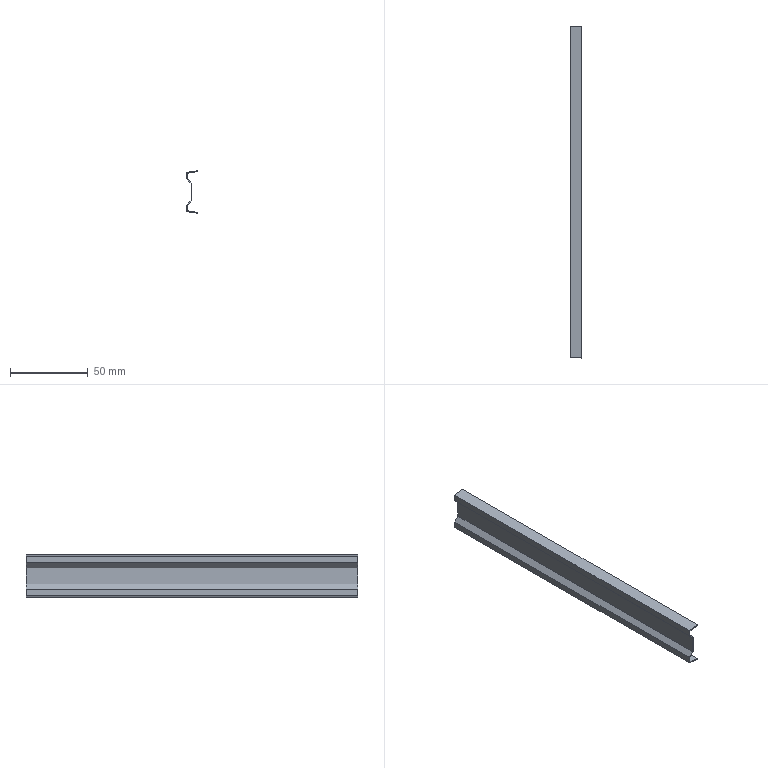Part | NX | features RETAINER-2_5003_009_C-SRH51Y22 2 | 1 solid | 18 faces | box 7.411 x 212.9 x 27.26 mm | volume 5304 mm3 | plane 18
STEP:
#1=CARTESIAN_POINT('',(-205.075,-353.05,-73.9));
#2=VERTEX_POINT('',#1);
#3=CARTESIAN_POINT('',(-197.747,-353.05,-72.87));
#4=VERTEX_POINT('',#3);
#5=CARTESIAN_POINT('',(-205.075,-353.05,-73.9));
#6=DIRECTION('',(0.9903,0.,0.1392));
#7=VECTOR('',#6,1000.);
#8=LINE('',#5,#7);
#9=EDGE_CURVE('',#2,#4,#8,.T.);
#10=ORIENTED_EDGE('',*,*,#9,.T.);
#11=CARTESIAN_POINT('',(-197.747,-140.15,-72.87));
#12=VERTEX_POINT('',#11);
#13=CARTESIAN_POINT('',(-197.747,-140.15,-72.87));
#14=DIRECTION('',(0.,-1.,0.));
#15=VECTOR('',#14,1000.);
#16=LINE('',#13,#15);
#17=EDGE_CURVE('',#12,#4,#16,.T.);
#18=ORIENTED_EDGE('',*,*,#17,.F.);
#19=CARTESIAN_POINT('',(-205.075,-140.15,-73.9));
#20=VERTEX_POINT('',#19);
#21=CARTESIAN_POINT('',(-205.075,-140.15,-73.9));
#22=DIRECTION('',(0.9903,0.,0.1392));
#23=VECTOR('',#22,1000.);
#24=LINE('',#21,#23);
#25=EDGE_CURVE('',#20,#12,#24,.T.);
#26=ORIENTED_EDGE('',*,*,#25,.F.);
#27=CARTESIAN_POINT('',(-205.075,-140.15,-73.9));
#28=DIRECTION('',(0.,-1.,0.));
#29=VECTOR('',#28,1000.);
#30=LINE('',#27,#29);
#31=EDGE_CURVE('',#20,#2,#30,.T.);
#32=ORIENTED_EDGE('',*,*,#31,.T.);
#33=EDGE_LOOP('',(#10,#18,#26,#32));
#34=FACE_BOUND('',#33,.T.);
#35=CARTESIAN_POINT('',(-205.075,-140.15,-73.9));
#36=DIRECTION('',(0.1392,0.,-0.9903));
#37=DIRECTION('',(-0.9903,0.,-0.1392));
#38=AXIS2_PLACEMENT_3D('',#35,#36,#37);
#39=PLANE('',#38);
#40=ADVANCED_FACE('',(#34),#39,.F.);
#41=CARTESIAN_POINT('',(-197.664,-353.05,-73.464));
#42=VERTEX_POINT('',#41);
#43=CARTESIAN_POINT('',(-197.747,-353.05,-72.87));
#44=DIRECTION('',(0.1392,0.,-0.9903));
#45=VECTOR('',#44,1000.);
#46=LINE('',#43,#45);
#47=EDGE_CURVE('',#4,#42,#46,.T.);
#48=ORIENTED_EDGE('',*,*,#47,.T.);
#49=CARTESIAN_POINT('',(-197.664,-140.15,-73.464));
#50=VERTEX_POINT('',#49);
#51=CARTESIAN_POINT('',(-197.664,-140.15,-73.464));
#52=DIRECTION('',(0.,-1.,0.));
#53=VECTOR('',#52,1000.);
#54=LINE('',#51,#53);
#55=EDGE_CURVE('',#50,#42,#54,.T.);
#56=ORIENTED_EDGE('',*,*,#55,.F.);
#57=CARTESIAN_POINT('',(-197.747,-140.15,-72.87));
#58=DIRECTION('',(0.1392,0.,-0.9903));
#59=VECTOR('',#58,1000.);
#60=LINE('',#57,#59);
#61=EDGE_CURVE('',#12,#50,#60,.T.);
#62=ORIENTED_EDGE('',*,*,#61,.F.);
#63=ORIENTED_EDGE('',*,*,#17,.T.);
#64=EDGE_LOOP('',(#48,#56,#62,#63));
#65=FACE_BOUND('',#64,.T.);
#66=CARTESIAN_POINT('',(-197.747,-140.15,-72.87));
#67=DIRECTION('',(-0.9903,0.,-0.1392));
#68=DIRECTION('',(-0.1392,0.,0.9903));
#69=AXIS2_PLACEMENT_3D('',#66,#67,#68);
#70=PLANE('',#69);
#71=ADVANCED_FACE('',(#65),#70,.F.);
#72=CARTESIAN_POINT('',(-204.475,-353.05,-74.422));
#73=VERTEX_POINT('',#72);
#74=CARTESIAN_POINT('',(-204.475,-353.05,-74.422));
#75=DIRECTION('',(-0.9903,0.,-0.1392));
#76=VECTOR('',#75,1000.);
#77=LINE('',#74,#76);
#78=EDGE_CURVE('',#42,#73,#77,.T.);
#79=ORIENTED_EDGE('',*,*,#78,.T.);
#80=CARTESIAN_POINT('',(-204.475,-140.15,-74.422));
#81=VERTEX_POINT('',#80);
#82=CARTESIAN_POINT('',(-204.475,-140.15,-74.422));
#83=DIRECTION('',(0.,-1.,0.));
#84=VECTOR('',#83,1000.);
#85=LINE('',#82,#84);
#86=EDGE_CURVE('',#81,#73,#85,.T.);
#87=ORIENTED_EDGE('',*,*,#86,.F.);
#88=CARTESIAN_POINT('',(-204.475,-140.15,-74.422));
#89=DIRECTION('',(-0.9903,0.,-0.1392));
#90=VECTOR('',#89,1000.);
#91=LINE('',#88,#90);
#92=EDGE_CURVE('',#50,#81,#91,.T.);
#93=ORIENTED_EDGE('',*,*,#92,.F.);
#94=ORIENTED_EDGE('',*,*,#55,.T.);
#95=EDGE_LOOP('',(#79,#87,#93,#94));
#96=FACE_BOUND('',#95,.T.);
#97=CARTESIAN_POINT('',(-204.475,-140.15,-74.422));
#98=DIRECTION('',(-0.1392,0.,0.9903));
#99=DIRECTION('',(0.9903,0.,0.1392));
#100=AXIS2_PLACEMENT_3D('',#97,#98,#99);
#101=PLANE('',#100);
#102=ADVANCED_FACE('',(#96),#101,.F.);
#103=CARTESIAN_POINT('',(-204.475,-353.05,-77.751));
#104=VERTEX_POINT('',#103);
#105=CARTESIAN_POINT('',(-204.475,-353.05,-74.422));
#106=DIRECTION('',(0.,0.,-1.));
#107=VECTOR('',#106,1000.);
#108=LINE('',#105,#107);
#109=EDGE_CURVE('',#73,#104,#108,.T.);
#110=ORIENTED_EDGE('',*,*,#109,.T.);
#111=CARTESIAN_POINT('',(-204.475,-140.15,-77.751));
#112=VERTEX_POINT('',#111);
#113=CARTESIAN_POINT('',(-204.475,-140.15,-77.751));
#114=DIRECTION('',(0.,-1.,0.));
#115=VECTOR('',#114,1000.);
#116=LINE('',#113,#115);
#117=EDGE_CURVE('',#112,#104,#116,.T.);
#118=ORIENTED_EDGE('',*,*,#117,.F.);
#119=CARTESIAN_POINT('',(-204.475,-140.15,-74.422));
#120=DIRECTION('',(0.,0.,-1.));
#121=VECTOR('',#120,1000.);
#122=LINE('',#119,#121);
#123=EDGE_CURVE('',#81,#112,#122,.T.);
#124=ORIENTED_EDGE('',*,*,#123,.F.);
#125=ORIENTED_EDGE('',*,*,#86,.T.);
#126=EDGE_LOOP('',(#110,#118,#124,#125));
#127=FACE_BOUND('',#126,.T.);
#128=CARTESIAN_POINT('',(-204.475,-140.15,-74.422));
#129=DIRECTION('',(-1.,0.,0.));
#130=DIRECTION('',(0.,-1.,0.));
#131=AXIS2_PLACEMENT_3D('',#128,#129,#130);
#132=PLANE('',#131);
#133=ADVANCED_FACE('',(#127),#132,.F.);
#134=CARTESIAN_POINT('',(-201.375,-353.05,-80.851));
#135=VERTEX_POINT('',#134);
#136=CARTESIAN_POINT('',(-204.475,-353.05,-77.751));
#137=DIRECTION('',(0.7071,0.,-0.7071));
#138=VECTOR('',#137,1000.);
#139=LINE('',#136,#138);
#140=EDGE_CURVE('',#104,#135,#139,.T.);
#141=ORIENTED_EDGE('',*,*,#140,.T.);
#142=CARTESIAN_POINT('',(-201.375,-140.15,-80.851));
#143=VERTEX_POINT('',#142);
#144=CARTESIAN_POINT('',(-201.375,-140.15,-80.851));
#145=DIRECTION('',(0.,-1.,0.));
#146=VECTOR('',#145,1000.);
#147=LINE('',#144,#146);
#148=EDGE_CURVE('',#143,#135,#147,.T.);
#149=ORIENTED_EDGE('',*,*,#148,.F.);
#150=CARTESIAN_POINT('',(-204.475,-140.15,-77.751));
#151=DIRECTION('',(0.7071,0.,-0.7071));
#152=VECTOR('',#151,1000.);
#153=LINE('',#150,#152);
#154=EDGE_CURVE('',#112,#143,#153,.T.);
#155=ORIENTED_EDGE('',*,*,#154,.F.);
#156=ORIENTED_EDGE('',*,*,#117,.T.);
#157=EDGE_LOOP('',(#141,#149,#155,#156));
#158=FACE_BOUND('',#157,.T.);
#159=CARTESIAN_POINT('',(-204.475,-140.15,-77.751));
#160=DIRECTION('',(-0.7071,0.,-0.7071));
#161=DIRECTION('',(-0.7071,0.,0.7071));
#162=AXIS2_PLACEMENT_3D('',#159,#160,#161);
#163=PLANE('',#162);
#164=ADVANCED_FACE('',(#158),#163,.F.);
#165=CARTESIAN_POINT('',(-201.375,-353.05,-92.149));
#166=VERTEX_POINT('',#165);
#167=CARTESIAN_POINT('',(-201.375,-353.05,-92.149));
#168=DIRECTION('',(0.,0.,-1.));
#169=VECTOR('',#168,1000.);
#170=LINE('',#167,#169);
#171=EDGE_CURVE('',#135,#166,#170,.T.);
#172=ORIENTED_EDGE('',*,*,#171,.T.);
#173=CARTESIAN_POINT('',(-201.375,-140.15,-92.149));
#174=VERTEX_POINT('',#173);
#175=CARTESIAN_POINT('',(-201.375,-140.15,-92.149));
#176=DIRECTION('',(0.,-1.,0.));
#177=VECTOR('',#176,1000.);
#178=LINE('',#175,#177);
#179=EDGE_CURVE('',#174,#166,#178,.T.);
#180=ORIENTED_EDGE('',*,*,#179,.F.);
#181=CARTESIAN_POINT('',(-201.375,-140.15,-92.149));
#182=DIRECTION('',(0.,0.,-1.));
#183=VECTOR('',#182,1000.);
#184=LINE('',#181,#183);
#185=EDGE_CURVE('',#143,#174,#184,.T.);
#186=ORIENTED_EDGE('',*,*,#185,.F.);
#187=ORIENTED_EDGE('',*,*,#148,.T.);
#188=EDGE_LOOP('',(#172,#180,#186,#187));
#189=FACE_BOUND('',#188,.T.);
#190=CARTESIAN_POINT('',(-201.375,-140.15,-92.149));
#191=DIRECTION('',(-1.,0.,0.));
#192=DIRECTION('',(0.,-1.,0.));
#193=AXIS2_PLACEMENT_3D('',#190,#191,#192);
#194=PLANE('',#193);
#195=ADVANCED_FACE('',(#189),#194,.F.);
#196=CARTESIAN_POINT('',(-204.475,-353.05,-95.249));
#197=VERTEX_POINT('',#196);
#198=CARTESIAN_POINT('',(-204.475,-353.05,-95.249));
#199=DIRECTION('',(-0.7071,0.,-0.7071));
#200=VECTOR('',#199,1000.);
#201=LINE('',#198,#200);
#202=EDGE_CURVE('',#166,#197,#201,.T.);
#203=ORIENTED_EDGE('',*,*,#202,.T.);
#204=CARTESIAN_POINT('',(-204.475,-140.15,-95.249));
#205=VERTEX_POINT('',#204);
#206=CARTESIAN_POINT('',(-204.475,-140.15,-95.249));
#207=DIRECTION('',(0.,-1.,0.));
#208=VECTOR('',#207,1000.);
#209=LINE('',#206,#208);
#210=EDGE_CURVE('',#205,#197,#209,.T.);
#211=ORIENTED_EDGE('',*,*,#210,.F.);
#212=CARTESIAN_POINT('',(-204.475,-140.15,-95.249));
#213=DIRECTION('',(-0.7071,0.,-0.7071));
#214=VECTOR('',#213,1000.);
#215=LINE('',#212,#214);
#216=EDGE_CURVE('',#174,#205,#215,.T.);
#217=ORIENTED_EDGE('',*,*,#216,.F.);
#218=ORIENTED_EDGE('',*,*,#179,.T.);
#219=EDGE_LOOP('',(#203,#211,#217,#218));
#220=FACE_BOUND('',#219,.T.);
#221=CARTESIAN_POINT('',(-204.475,-140.15,-95.249));
#222=DIRECTION('',(-0.7071,0.,0.7071));
#223=DIRECTION('',(0.7071,0.,0.7071));
#224=AXIS2_PLACEMENT_3D('',#221,#222,#223);
#225=PLANE('',#224);
#226=ADVANCED_FACE('',(#220),#225,.F.);
#227=CARTESIAN_POINT('',(-204.475,-353.05,-98.578));
#228=VERTEX_POINT('',#227);
#229=CARTESIAN_POINT('',(-204.475,-353.05,-98.578));
#230=DIRECTION('',(0.,0.,-1.));
#231=VECTOR('',#230,1000.);
#232=LINE('',#229,#231);
#233=EDGE_CURVE('',#197,#228,#232,.T.);
#234=ORIENTED_EDGE('',*,*,#233,.T.);
#235=CARTESIAN_POINT('',(-204.475,-140.15,-98.578));
#236=VERTEX_POINT('',#235);
#237=CARTESIAN_POINT('',(-204.475,-140.15,-98.578));
#238=DIRECTION('',(0.,-1.,0.));
#239=VECTOR('',#238,1000.);
#240=LINE('',#237,#239);
#241=EDGE_CURVE('',#236,#228,#240,.T.);
#242=ORIENTED_EDGE('',*,*,#241,.F.);
#243=CARTESIAN_POINT('',(-204.475,-140.15,-98.578));
#244=DIRECTION('',(0.,0.,-1.));
#245=VECTOR('',#244,1000.);
#246=LINE('',#243,#245);
#247=EDGE_CURVE('',#205,#236,#246,.T.);
#248=ORIENTED_EDGE('',*,*,#247,.F.);
#249=ORIENTED_EDGE('',*,*,#210,.T.);
#250=EDGE_LOOP('',(#234,#242,#248,#249));
#251=FACE_BOUND('',#250,.T.);
#252=CARTESIAN_POINT('',(-204.475,-140.15,-98.578));
#253=DIRECTION('',(-1.,0.,0.));
#254=DIRECTION('',(0.,-1.,0.));
#255=AXIS2_PLACEMENT_3D('',#252,#253,#254);
#256=PLANE('',#255);
#257=ADVANCED_FACE('',(#251),#256,.F.);
#258=CARTESIAN_POINT('',(-197.664,-353.05,-99.536));
#259=VERTEX_POINT('',#258);
#260=CARTESIAN_POINT('',(-204.475,-353.05,-98.578));
#261=DIRECTION('',(0.9903,0.,-0.1392));
#262=VECTOR('',#261,1000.);
#263=LINE('',#260,#262);
#264=EDGE_CURVE('',#228,#259,#263,.T.);
#265=ORIENTED_EDGE('',*,*,#264,.T.);
#266=CARTESIAN_POINT('',(-197.664,-140.15,-99.536));
#267=VERTEX_POINT('',#266);
#268=CARTESIAN_POINT('',(-197.664,-140.15,-99.536));
#269=DIRECTION('',(0.,-1.,0.));
#270=VECTOR('',#269,1000.);
#271=LINE('',#268,#270);
#272=EDGE_CURVE('',#267,#259,#271,.T.);
#273=ORIENTED_EDGE('',*,*,#272,.F.);
#274=CARTESIAN_POINT('',(-204.475,-140.15,-98.578));
#275=DIRECTION('',(0.9903,0.,-0.1392));
#276=VECTOR('',#275,1000.);
#277=LINE('',#274,#276);
#278=EDGE_CURVE('',#236,#267,#277,.T.);
#279=ORIENTED_EDGE('',*,*,#278,.F.);
#280=ORIENTED_EDGE('',*,*,#241,.T.);
#281=EDGE_LOOP('',(#265,#273,#279,#280));
#282=FACE_BOUND('',#281,.T.);
#283=CARTESIAN_POINT('',(-204.475,-140.15,-98.578));
#284=DIRECTION('',(-0.1392,0.,-0.9903));
#285=DIRECTION('',(-0.9903,0.,0.1392));
#286=AXIS2_PLACEMENT_3D('',#283,#284,#285);
#287=PLANE('',#286);
#288=ADVANCED_FACE('',(#282),#287,.F.);
#289=CARTESIAN_POINT('',(-197.747,-353.05,-100.13));
#290=VERTEX_POINT('',#289);
#291=CARTESIAN_POINT('',(-197.664,-353.05,-99.536));
#292=DIRECTION('',(-0.1392,0.,-0.9903));
#293=VECTOR('',#292,1000.);
#294=LINE('',#291,#293);
#295=EDGE_CURVE('',#259,#290,#294,.T.);
#296=ORIENTED_EDGE('',*,*,#295,.T.);
#297=CARTESIAN_POINT('',(-197.747,-140.15,-100.13));
#298=VERTEX_POINT('',#297);
#299=CARTESIAN_POINT('',(-197.747,-140.15,-100.13));
#300=DIRECTION('',(0.,-1.,0.));
#301=VECTOR('',#300,1000.);
#302=LINE('',#299,#301);
#303=EDGE_CURVE('',#298,#290,#302,.T.);
#304=ORIENTED_EDGE('',*,*,#303,.F.);
#305=CARTESIAN_POINT('',(-197.664,-140.15,-99.536));
#306=DIRECTION('',(-0.1392,0.,-0.9903));
#307=VECTOR('',#306,1000.);
#308=LINE('',#305,#307);
#309=EDGE_CURVE('',#267,#298,#308,.T.);
#310=ORIENTED_EDGE('',*,*,#309,.F.);
#311=ORIENTED_EDGE('',*,*,#272,.T.);
#312=EDGE_LOOP('',(#296,#304,#310,#311));
#313=FACE_BOUND('',#312,.T.);
#314=CARTESIAN_POINT('',(-197.664,-140.15,-99.536));
#315=DIRECTION('',(-0.9903,0.,0.1392));
#316=DIRECTION('',(0.1392,0.,0.9903));
#317=AXIS2_PLACEMENT_3D('',#314,#315,#316);
#318=PLANE('',#317);
#319=ADVANCED_FACE('',(#313),#318,.F.);
#320=CARTESIAN_POINT('',(-205.075,-353.05,-99.1));
#321=VERTEX_POINT('',#320);
#322=CARTESIAN_POINT('',(-205.075,-353.05,-99.1));
#323=DIRECTION('',(-0.9903,0.,0.1392));
#324=VECTOR('',#323,1000.);
#325=LINE('',#322,#324);
#326=EDGE_CURVE('',#290,#321,#325,.T.);
#327=ORIENTED_EDGE('',*,*,#326,.T.);
#328=CARTESIAN_POINT('',(-205.075,-140.15,-99.1));
#329=VERTEX_POINT('',#328);
#330=CARTESIAN_POINT('',(-205.075,-140.15,-99.1));
#331=DIRECTION('',(0.,-1.,0.));
#332=VECTOR('',#331,1000.);
#333=LINE('',#330,#332);
#334=EDGE_CURVE('',#329,#321,#333,.T.);
#335=ORIENTED_EDGE('',*,*,#334,.F.);
#336=CARTESIAN_POINT('',(-205.075,-140.15,-99.1));
#337=DIRECTION('',(-0.9903,0.,0.1392));
#338=VECTOR('',#337,1000.);
#339=LINE('',#336,#338);
#340=EDGE_CURVE('',#298,#329,#339,.T.);
#341=ORIENTED_EDGE('',*,*,#340,.F.);
#342=ORIENTED_EDGE('',*,*,#303,.T.);
#343=EDGE_LOOP('',(#327,#335,#341,#342));
#344=FACE_BOUND('',#343,.T.);
#345=CARTESIAN_POINT('',(-205.075,-140.15,-99.1));
#346=DIRECTION('',(0.1392,0.,0.9903));
#347=DIRECTION('',(0.9903,0.,-0.1392));
#348=AXIS2_PLACEMENT_3D('',#345,#346,#347);
#349=PLANE('',#348);
#350=ADVANCED_FACE('',(#344),#349,.F.);
#351=CARTESIAN_POINT('',(-205.075,-353.05,-95.));
#352=VERTEX_POINT('',#351);
#353=CARTESIAN_POINT('',(-205.075,-353.05,-99.1));
#354=DIRECTION('',(0.,0.,1.));
#355=VECTOR('',#354,1000.);
#356=LINE('',#353,#355);
#357=EDGE_CURVE('',#321,#352,#356,.T.);
#358=ORIENTED_EDGE('',*,*,#357,.T.);
#359=CARTESIAN_POINT('',(-205.075,-140.15,-95.));
#360=VERTEX_POINT('',#359);
#361=CARTESIAN_POINT('',(-205.075,-140.15,-95.));
#362=DIRECTION('',(0.,-1.,0.));
#363=VECTOR('',#362,1000.);
#364=LINE('',#361,#363);
#365=EDGE_CURVE('',#360,#352,#364,.T.);
#366=ORIENTED_EDGE('',*,*,#365,.F.);
#367=CARTESIAN_POINT('',(-205.075,-140.15,-99.1));
#368=DIRECTION('',(0.,0.,1.));
#369=VECTOR('',#368,1000.);
#370=LINE('',#367,#369);
#371=EDGE_CURVE('',#329,#360,#370,.T.);
#372=ORIENTED_EDGE('',*,*,#371,.F.);
#373=ORIENTED_EDGE('',*,*,#334,.T.);
#374=EDGE_LOOP('',(#358,#366,#372,#373));
#375=FACE_BOUND('',#374,.T.);
#376=CARTESIAN_POINT('',(-205.075,-140.15,-99.1));
#377=DIRECTION('',(1.,0.,0.));
#378=DIRECTION('',(0.,0.,-1.));
#379=AXIS2_PLACEMENT_3D('',#376,#377,#378);
#380=PLANE('',#379);
#381=ADVANCED_FACE('',(#375),#380,.F.);
#382=CARTESIAN_POINT('',(-201.975,-353.05,-91.9));
#383=VERTEX_POINT('',#382);
#384=CARTESIAN_POINT('',(-205.075,-353.05,-95.));
#385=DIRECTION('',(0.7071,0.,0.7071));
#386=VECTOR('',#385,1000.);
#387=LINE('',#384,#386);
#388=EDGE_CURVE('',#352,#383,#387,.T.);
#389=ORIENTED_EDGE('',*,*,#388,.T.);
#390=CARTESIAN_POINT('',(-201.975,-140.15,-91.9));
#391=VERTEX_POINT('',#390);
#392=CARTESIAN_POINT('',(-201.975,-140.15,-91.9));
#393=DIRECTION('',(0.,-1.,0.));
#394=VECTOR('',#393,1000.);
#395=LINE('',#392,#394);
#396=EDGE_CURVE('',#391,#383,#395,.T.);
#397=ORIENTED_EDGE('',*,*,#396,.F.);
#398=CARTESIAN_POINT('',(-205.075,-140.15,-95.));
#399=DIRECTION('',(0.7071,0.,0.7071));
#400=VECTOR('',#399,1000.);
#401=LINE('',#398,#400);
#402=EDGE_CURVE('',#360,#391,#401,.T.);
#403=ORIENTED_EDGE('',*,*,#402,.F.);
#404=ORIENTED_EDGE('',*,*,#365,.T.);
#405=EDGE_LOOP('',(#389,#397,#403,#404));
#406=FACE_BOUND('',#405,.T.);
#407=CARTESIAN_POINT('',(-205.075,-140.15,-95.));
#408=DIRECTION('',(0.7071,0.,-0.7071));
#409=DIRECTION('',(-0.7071,0.,-0.7071));
#410=AXIS2_PLACEMENT_3D('',#407,#408,#409);
#411=PLANE('',#410);
#412=ADVANCED_FACE('',(#406),#411,.F.);
#413=CARTESIAN_POINT('',(-201.975,-353.05,-81.1));
#414=VERTEX_POINT('',#413);
#415=CARTESIAN_POINT('',(-201.975,-353.05,-91.9));
#416=DIRECTION('',(0.,0.,1.));
#417=VECTOR('',#416,1000.);
#418=LINE('',#415,#417);
#419=EDGE_CURVE('',#383,#414,#418,.T.);
#420=ORIENTED_EDGE('',*,*,#419,.T.);
#421=CARTESIAN_POINT('',(-201.975,-140.15,-81.1));
#422=VERTEX_POINT('',#421);
#423=CARTESIAN_POINT('',(-201.975,-140.15,-81.1));
#424=DIRECTION('',(0.,-1.,0.));
#425=VECTOR('',#424,1000.);
#426=LINE('',#423,#425);
#427=EDGE_CURVE('',#422,#414,#426,.T.);
#428=ORIENTED_EDGE('',*,*,#427,.F.);
#429=CARTESIAN_POINT('',(-201.975,-140.15,-91.9));
#430=DIRECTION('',(0.,0.,1.));
#431=VECTOR('',#430,1000.);
#432=LINE('',#429,#431);
#433=EDGE_CURVE('',#391,#422,#432,.T.);
#434=ORIENTED_EDGE('',*,*,#433,.F.);
#435=ORIENTED_EDGE('',*,*,#396,.T.);
#436=EDGE_LOOP('',(#420,#428,#434,#435));
#437=FACE_BOUND('',#436,.T.);
#438=CARTESIAN_POINT('',(-201.975,-140.15,-91.9));
#439=DIRECTION('',(1.,0.,0.));
#440=DIRECTION('',(0.,0.,-1.));
#441=AXIS2_PLACEMENT_3D('',#438,#439,#440);
#442=PLANE('',#441);
#443=ADVANCED_FACE('',(#437),#442,.F.);
#444=CARTESIAN_POINT('',(-205.075,-353.05,-78.));
#445=VERTEX_POINT('',#444);
#446=CARTESIAN_POINT('',(-205.075,-353.05,-78.));
#447=DIRECTION('',(-0.7071,0.,0.7071));
#448=VECTOR('',#447,1000.);
#449=LINE('',#446,#448);
#450=EDGE_CURVE('',#414,#445,#449,.T.);
#451=ORIENTED_EDGE('',*,*,#450,.T.);
#452=CARTESIAN_POINT('',(-205.075,-140.15,-78.));
#453=VERTEX_POINT('',#452);
#454=CARTESIAN_POINT('',(-205.075,-140.15,-78.));
#455=DIRECTION('',(0.,-1.,0.));
#456=VECTOR('',#455,1000.);
#457=LINE('',#454,#456);
#458=EDGE_CURVE('',#453,#445,#457,.T.);
#459=ORIENTED_EDGE('',*,*,#458,.F.);
#460=CARTESIAN_POINT('',(-205.075,-140.15,-78.));
#461=DIRECTION('',(-0.7071,0.,0.7071));
#462=VECTOR('',#461,1000.);
#463=LINE('',#460,#462);
#464=EDGE_CURVE('',#422,#453,#463,.T.);
#465=ORIENTED_EDGE('',*,*,#464,.F.);
#466=ORIENTED_EDGE('',*,*,#427,.T.);
#467=EDGE_LOOP('',(#451,#459,#465,#466));
#468=FACE_BOUND('',#467,.T.);
#469=CARTESIAN_POINT('',(-205.075,-140.15,-78.));
#470=DIRECTION('',(0.7071,0.,0.7071));
#471=DIRECTION('',(0.7071,0.,-0.7071));
#472=AXIS2_PLACEMENT_3D('',#469,#470,#471);
#473=PLANE('',#472);
#474=ADVANCED_FACE('',(#468),#473,.F.);
#475=CARTESIAN_POINT('',(-205.075,-353.05,-73.9));
#476=DIRECTION('',(0.,0.,1.));
#477=VECTOR('',#476,1000.);
#478=LINE('',#475,#477);
#479=EDGE_CURVE('',#445,#2,#478,.T.);
#480=ORIENTED_EDGE('',*,*,#479,.T.);
#481=ORIENTED_EDGE('',*,*,#31,.F.);
#482=CARTESIAN_POINT('',(-205.075,-140.15,-73.9));
#483=DIRECTION('',(0.,0.,1.));
#484=VECTOR('',#483,1000.);
#485=LINE('',#482,#484);
#486=EDGE_CURVE('',#453,#20,#485,.T.);
#487=ORIENTED_EDGE('',*,*,#486,.F.);
#488=ORIENTED_EDGE('',*,*,#458,.T.);
#489=EDGE_LOOP('',(#480,#481,#487,#488));
#490=FACE_BOUND('',#489,.T.);
#491=CARTESIAN_POINT('',(-205.075,-140.15,-73.9));
#492=DIRECTION('',(1.,0.,0.));
#493=DIRECTION('',(0.,0.,-1.));
#494=AXIS2_PLACEMENT_3D('',#491,#492,#493);
#495=PLANE('',#494);
#496=ADVANCED_FACE('',(#490),#495,.F.);
#497=ORIENTED_EDGE('',*,*,#25,.T.);
#498=ORIENTED_EDGE('',*,*,#61,.T.);
#499=ORIENTED_EDGE('',*,*,#92,.T.);
#500=ORIENTED_EDGE('',*,*,#123,.T.);
#501=ORIENTED_EDGE('',*,*,#154,.T.);
#502=ORIENTED_EDGE('',*,*,#185,.T.);
#503=ORIENTED_EDGE('',*,*,#216,.T.);
#504=ORIENTED_EDGE('',*,*,#247,.T.);
#505=ORIENTED_EDGE('',*,*,#278,.T.);
#506=ORIENTED_EDGE('',*,*,#309,.T.);
#507=ORIENTED_EDGE('',*,*,#340,.T.);
#508=ORIENTED_EDGE('',*,*,#371,.T.);
#509=ORIENTED_EDGE('',*,*,#402,.T.);
#510=ORIENTED_EDGE('',*,*,#433,.T.);
#511=ORIENTED_EDGE('',*,*,#464,.T.);
#512=ORIENTED_EDGE('',*,*,#486,.T.);
#513=EDGE_LOOP('',(#497,#498,#499,#500,#501,#502,#503,#504,#505,#506,#507,#508,#509,#510,#511,#512));
#514=FACE_BOUND('',#513,.T.);
#515=CARTESIAN_POINT('',(-201.375,-140.15,-86.5));
#516=DIRECTION('',(0.,1.,0.));
#517=DIRECTION('',(-1.,0.,0.));
#518=AXIS2_PLACEMENT_3D('',#515,#516,#517);
#519=PLANE('',#518);
#520=ADVANCED_FACE('',(#514),#519,.T.);
#521=ORIENTED_EDGE('',*,*,#9,.F.);
#522=ORIENTED_EDGE('',*,*,#479,.F.);
#523=ORIENTED_EDGE('',*,*,#450,.F.);
#524=ORIENTED_EDGE('',*,*,#419,.F.);
#525=ORIENTED_EDGE('',*,*,#388,.F.);
#526=ORIENTED_EDGE('',*,*,#357,.F.);
#527=ORIENTED_EDGE('',*,*,#326,.F.);
#528=ORIENTED_EDGE('',*,*,#295,.F.);
#529=ORIENTED_EDGE('',*,*,#264,.F.);
#530=ORIENTED_EDGE('',*,*,#233,.F.);
#531=ORIENTED_EDGE('',*,*,#202,.F.);
#532=ORIENTED_EDGE('',*,*,#171,.F.);
#533=ORIENTED_EDGE('',*,*,#140,.F.);
#534=ORIENTED_EDGE('',*,*,#109,.F.);
#535=ORIENTED_EDGE('',*,*,#78,.F.);
#536=ORIENTED_EDGE('',*,*,#47,.F.);
#537=EDGE_LOOP('',(#521,#522,#523,#524,#525,#526,#527,#528,#529,#530,#531,#532,#533,#534,#535,#536));
#538=FACE_BOUND('',#537,.T.);
#539=CARTESIAN_POINT('',(-201.375,-353.05,-86.5));
#540=DIRECTION('',(0.,1.,0.));
#541=DIRECTION('',(-1.,0.,0.));
#542=AXIS2_PLACEMENT_3D('',#539,#540,#541);
#543=PLANE('',#542);
#544=ADVANCED_FACE('',(#538),#543,.F.);
#545=CLOSED_SHELL('',(#40,#71,#102,#133,#164,#195,#226,#257,#288,#319,#350,#381,#412,#443,#474,#496,#520,#544));
#546=MANIFOLD_SOLID_BREP('',#545);
#547=(LENGTH_UNIT()NAMED_UNIT(*)SI_UNIT(.MILLI.,.METRE.));
#548=UNCERTAINTY_MEASURE_WITH_UNIT(LENGTH_MEASURE(0.00001),#547,'','');
#549=(NAMED_UNIT(*)PLANE_ANGLE_UNIT()SI_UNIT($,.RADIAN.));
#550=(NAMED_UNIT(*)SI_UNIT($,.STERADIAN.)SOLID_ANGLE_UNIT());
#551=(GEOMETRIC_REPRESENTATION_CONTEXT(3)GLOBAL_UNCERTAINTY_ASSIGNED_CONTEXT((#548))GLOBAL_UNIT_ASSIGNED_CONTEXT((#547,#549,#550))REPRESENTATION_CONTEXT('',''));
#552=ADVANCED_BREP_SHAPE_REPRESENTATION('',(#546),#551);